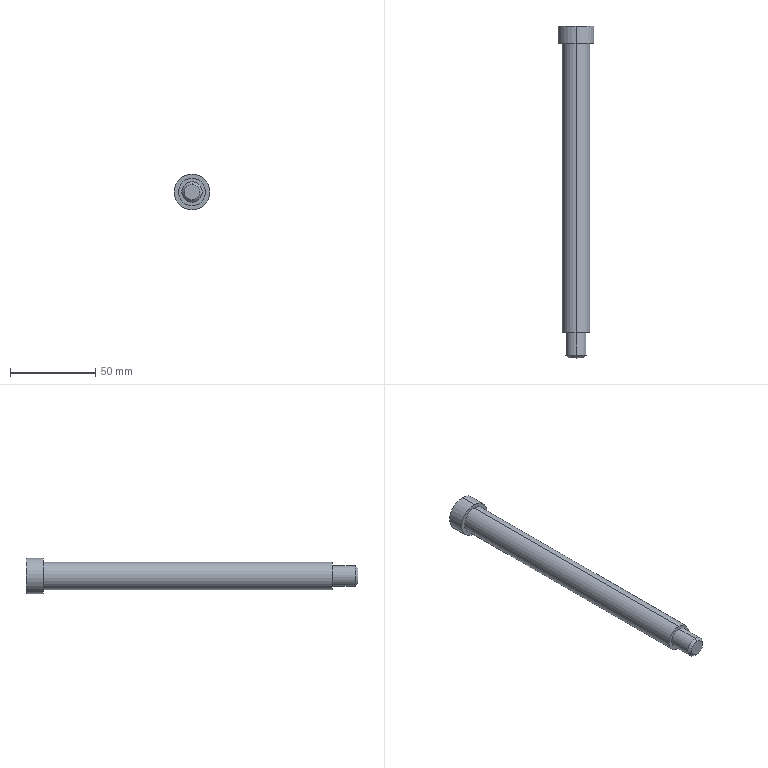Part | Creo | 1 solid | 19 faces | box 21 x 195 x 21 mm | volume 38969 mm3 | plane 11 | cylinder 6 | cone 2 | commonest cylinder face diameters 12 x2 16 x2 21 x2
STEP:
#1=CARTESIAN_POINT('',(0.2584,548.92,-30.381));
#2=VERTEX_POINT('',#1);
#3=CARTESIAN_POINT('',(4.258,548.92,-32.691));
#4=VERTEX_POINT('',#3);
#5=CARTESIAN_POINT('',(0.2584,548.92,-30.381));
#6=DIRECTION('',(0.866,0.,-0.5));
#7=VECTOR('',#6,4.619);
#8=LINE('',#5,#7);
#9=EDGE_CURVE('',#2,#4,#8,.T.);
#10=ORIENTED_EDGE('',*,*,#9,.F.);
#11=CARTESIAN_POINT('',(-3.742,548.92,-32.691));
#12=VERTEX_POINT('',#11);
#13=CARTESIAN_POINT('',(-3.742,548.92,-32.691));
#14=DIRECTION('',(0.866,0.,0.5));
#15=VECTOR('',#14,4.619);
#16=LINE('',#13,#15);
#17=EDGE_CURVE('',#12,#2,#16,.T.);
#18=ORIENTED_EDGE('',*,*,#17,.F.);
#19=CARTESIAN_POINT('',(-3.742,548.92,-37.309));
#20=VERTEX_POINT('',#19);
#21=CARTESIAN_POINT('',(-3.742,548.92,-32.691));
#22=DIRECTION('',(0.,0.,-1.));
#23=VECTOR('',#22,4.619);
#24=LINE('',#21,#23);
#25=EDGE_CURVE('',#12,#20,#24,.T.);
#26=ORIENTED_EDGE('',*,*,#25,.T.);
#27=CARTESIAN_POINT('',(0.2584,548.92,-39.619));
#28=VERTEX_POINT('',#27);
#29=CARTESIAN_POINT('',(0.2584,548.92,-39.619));
#30=DIRECTION('',(-0.866,0.,0.5));
#31=VECTOR('',#30,4.619);
#32=LINE('',#29,#31);
#33=EDGE_CURVE('',#28,#20,#32,.T.);
#34=ORIENTED_EDGE('',*,*,#33,.F.);
#35=CARTESIAN_POINT('',(4.258,548.92,-37.309));
#36=VERTEX_POINT('',#35);
#37=CARTESIAN_POINT('',(4.258,548.92,-37.309));
#38=DIRECTION('',(-0.866,0.,-0.5));
#39=VECTOR('',#38,4.619);
#40=LINE('',#37,#39);
#41=EDGE_CURVE('',#36,#28,#40,.T.);
#42=ORIENTED_EDGE('',*,*,#41,.F.);
#43=CARTESIAN_POINT('',(4.258,548.92,-37.309));
#44=DIRECTION('',(0.,0.,1.));
#45=VECTOR('',#44,4.619);
#46=LINE('',#43,#45);
#47=EDGE_CURVE('',#36,#4,#46,.T.);
#48=ORIENTED_EDGE('',*,*,#47,.T.);
#49=EDGE_LOOP('',(#10,#18,#26,#34,#42,#48));
#50=FACE_OUTER_BOUND('',#49,.F.);
#51=CARTESIAN_POINT('',(0.2584,548.92,-35.));
#52=DIRECTION('',(0.,1.,0.));
#53=DIRECTION('',(0.,0.,1.));
#54=AXIS2_PLACEMENT_3D('',#51,#52,#53);
#55=PLANE('',#54);
#56=ADVANCED_FACE('',(#50),#55,.T.);
#57=CARTESIAN_POINT('',(4.258,554.92,-32.691));
#58=VERTEX_POINT('',#57);
#59=CARTESIAN_POINT('',(4.258,548.92,-32.691));
#60=DIRECTION('',(0.,1.,0.));
#61=VECTOR('',#60,6.);
#62=LINE('',#59,#61);
#63=EDGE_CURVE('',#4,#58,#62,.T.);
#64=ORIENTED_EDGE('',*,*,#63,.T.);
#65=CARTESIAN_POINT('',(0.2584,554.92,-30.381));
#66=VERTEX_POINT('',#65);
#67=CARTESIAN_POINT('',(4.258,554.92,-32.691));
#68=DIRECTION('',(-0.866,0.,0.5));
#69=VECTOR('',#68,4.619);
#70=LINE('',#67,#69);
#71=EDGE_CURVE('',#58,#66,#70,.T.);
#72=ORIENTED_EDGE('',*,*,#71,.T.);
#73=CARTESIAN_POINT('',(0.2584,548.92,-30.381));
#74=DIRECTION('',(0.,1.,0.));
#75=VECTOR('',#74,6.);
#76=LINE('',#73,#75);
#77=EDGE_CURVE('',#2,#66,#76,.T.);
#78=ORIENTED_EDGE('',*,*,#77,.F.);
#79=ORIENTED_EDGE('',*,*,#9,.T.);
#80=EDGE_LOOP('',(#64,#72,#78,#79));
#81=FACE_OUTER_BOUND('',#80,.F.);
#82=CARTESIAN_POINT('',(0.2584,554.92,-30.381));
#83=DIRECTION('',(0.5,0.,0.866));
#84=DIRECTION('',(-0.866,0.,0.5));
#85=AXIS2_PLACEMENT_3D('',#82,#83,#84);
#86=PLANE('',#85);
#87=ADVANCED_FACE('',(#81),#86,.F.);
#88=CARTESIAN_POINT('',(4.258,554.92,-37.309));
#89=VERTEX_POINT('',#88);
#90=CARTESIAN_POINT('',(4.258,548.92,-37.309));
#91=DIRECTION('',(0.,1.,0.));
#92=VECTOR('',#91,6.);
#93=LINE('',#90,#92);
#94=EDGE_CURVE('',#36,#89,#93,.T.);
#95=ORIENTED_EDGE('',*,*,#94,.T.);
#96=CARTESIAN_POINT('',(4.258,554.92,-37.309));
#97=DIRECTION('',(0.,0.,1.));
#98=VECTOR('',#97,4.619);
#99=LINE('',#96,#98);
#100=EDGE_CURVE('',#89,#58,#99,.T.);
#101=ORIENTED_EDGE('',*,*,#100,.T.);
#102=ORIENTED_EDGE('',*,*,#63,.F.);
#103=ORIENTED_EDGE('',*,*,#47,.F.);
#104=EDGE_LOOP('',(#95,#101,#102,#103));
#105=FACE_OUTER_BOUND('',#104,.F.);
#106=CARTESIAN_POINT('',(4.258,554.92,-32.691));
#107=DIRECTION('',(1.,0.,0.));
#108=DIRECTION('',(0.,0.,1.));
#109=AXIS2_PLACEMENT_3D('',#106,#107,#108);
#110=PLANE('',#109);
#111=ADVANCED_FACE('',(#105),#110,.F.);
#112=CARTESIAN_POINT('',(0.2584,554.92,-39.619));
#113=VERTEX_POINT('',#112);
#114=CARTESIAN_POINT('',(0.2584,548.92,-39.619));
#115=DIRECTION('',(0.,1.,0.));
#116=VECTOR('',#115,6.);
#117=LINE('',#114,#116);
#118=EDGE_CURVE('',#28,#113,#117,.T.);
#119=ORIENTED_EDGE('',*,*,#118,.T.);
#120=CARTESIAN_POINT('',(0.2584,554.92,-39.619));
#121=DIRECTION('',(0.866,0.,0.5));
#122=VECTOR('',#121,4.619);
#123=LINE('',#120,#122);
#124=EDGE_CURVE('',#113,#89,#123,.T.);
#125=ORIENTED_EDGE('',*,*,#124,.T.);
#126=ORIENTED_EDGE('',*,*,#94,.F.);
#127=ORIENTED_EDGE('',*,*,#41,.T.);
#128=EDGE_LOOP('',(#119,#125,#126,#127));
#129=FACE_OUTER_BOUND('',#128,.F.);
#130=CARTESIAN_POINT('',(4.258,554.92,-37.309));
#131=DIRECTION('',(0.5,0.,-0.866));
#132=DIRECTION('',(0.866,0.,0.5));
#133=AXIS2_PLACEMENT_3D('',#130,#131,#132);
#134=PLANE('',#133);
#135=ADVANCED_FACE('',(#129),#134,.F.);
#136=CARTESIAN_POINT('',(-3.742,554.92,-37.309));
#137=VERTEX_POINT('',#136);
#138=CARTESIAN_POINT('',(-3.742,548.92,-37.309));
#139=DIRECTION('',(0.,1.,0.));
#140=VECTOR('',#139,6.);
#141=LINE('',#138,#140);
#142=EDGE_CURVE('',#20,#137,#141,.T.);
#143=ORIENTED_EDGE('',*,*,#142,.T.);
#144=CARTESIAN_POINT('',(-3.742,554.92,-37.309));
#145=DIRECTION('',(0.866,0.,-0.5));
#146=VECTOR('',#145,4.619);
#147=LINE('',#144,#146);
#148=EDGE_CURVE('',#137,#113,#147,.T.);
#149=ORIENTED_EDGE('',*,*,#148,.T.);
#150=ORIENTED_EDGE('',*,*,#118,.F.);
#151=ORIENTED_EDGE('',*,*,#33,.T.);
#152=EDGE_LOOP('',(#143,#149,#150,#151));
#153=FACE_OUTER_BOUND('',#152,.F.);
#154=CARTESIAN_POINT('',(0.2584,554.92,-39.619));
#155=DIRECTION('',(-0.5,0.,-0.866));
#156=DIRECTION('',(0.866,0.,-0.5));
#157=AXIS2_PLACEMENT_3D('',#154,#155,#156);
#158=PLANE('',#157);
#159=ADVANCED_FACE('',(#153),#158,.F.);
#160=CARTESIAN_POINT('',(-3.742,554.92,-32.691));
#161=VERTEX_POINT('',#160);
#162=CARTESIAN_POINT('',(-3.742,548.92,-32.691));
#163=DIRECTION('',(0.,1.,0.));
#164=VECTOR('',#163,6.);
#165=LINE('',#162,#164);
#166=EDGE_CURVE('',#12,#161,#165,.T.);
#167=ORIENTED_EDGE('',*,*,#166,.T.);
#168=CARTESIAN_POINT('',(-3.742,554.92,-32.691));
#169=DIRECTION('',(0.,0.,-1.));
#170=VECTOR('',#169,4.619);
#171=LINE('',#168,#170);
#172=EDGE_CURVE('',#161,#137,#171,.T.);
#173=ORIENTED_EDGE('',*,*,#172,.T.);
#174=ORIENTED_EDGE('',*,*,#142,.F.);
#175=ORIENTED_EDGE('',*,*,#25,.F.);
#176=EDGE_LOOP('',(#167,#173,#174,#175));
#177=FACE_OUTER_BOUND('',#176,.F.);
#178=CARTESIAN_POINT('',(-3.742,554.92,-37.309));
#179=DIRECTION('',(-1.,0.,0.));
#180=DIRECTION('',(0.,0.,-1.));
#181=AXIS2_PLACEMENT_3D('',#178,#179,#180);
#182=PLANE('',#181);
#183=ADVANCED_FACE('',(#177),#182,.F.);
#184=ORIENTED_EDGE('',*,*,#77,.T.);
#185=CARTESIAN_POINT('',(0.2584,554.92,-30.381));
#186=DIRECTION('',(-0.866,0.,-0.5));
#187=VECTOR('',#186,4.619);
#188=LINE('',#185,#187);
#189=EDGE_CURVE('',#66,#161,#188,.T.);
#190=ORIENTED_EDGE('',*,*,#189,.T.);
#191=ORIENTED_EDGE('',*,*,#166,.F.);
#192=ORIENTED_EDGE('',*,*,#17,.T.);
#193=EDGE_LOOP('',(#184,#190,#191,#192));
#194=FACE_OUTER_BOUND('',#193,.F.);
#195=CARTESIAN_POINT('',(-3.742,554.92,-32.691));
#196=DIRECTION('',(-0.5,0.,0.866));
#197=DIRECTION('',(-0.866,0.,-0.5));
#198=AXIS2_PLACEMENT_3D('',#195,#196,#197);
#199=PLANE('',#198);
#200=ADVANCED_FACE('',(#194),#199,.F.);
#201=CARTESIAN_POINT('',(0.2584,554.92,-24.5));
#202=VERTEX_POINT('',#201);
#203=CARTESIAN_POINT('',(0.2584,554.92,-45.5));
#204=VERTEX_POINT('',#203);
#205=CARTESIAN_POINT('',(0.2584,554.92,-35.));
#206=DIRECTION('',(0.,1.,0.));
#207=DIRECTION('',(0.,0.,1.));
#208=AXIS2_PLACEMENT_3D('',#205,#206,#207);
#209=CIRCLE('',#208,10.5);
#210=EDGE_CURVE('',#202,#204,#209,.T.);
#211=ORIENTED_EDGE('',*,*,#210,.F.);
#212=CARTESIAN_POINT('',(0.2584,554.92,-35.));
#213=DIRECTION('',(0.,1.,0.));
#214=DIRECTION('',(0.,0.,-1.));
#215=AXIS2_PLACEMENT_3D('',#212,#213,#214);
#216=CIRCLE('',#215,10.5);
#217=EDGE_CURVE('',#204,#202,#216,.T.);
#218=ORIENTED_EDGE('',*,*,#217,.F.);
#219=EDGE_LOOP('',(#211,#218));
#220=FACE_OUTER_BOUND('',#219,.F.);
#221=ORIENTED_EDGE('',*,*,#172,.F.);
#222=ORIENTED_EDGE('',*,*,#189,.F.);
#223=ORIENTED_EDGE('',*,*,#71,.F.);
#224=ORIENTED_EDGE('',*,*,#100,.F.);
#225=ORIENTED_EDGE('',*,*,#124,.F.);
#226=ORIENTED_EDGE('',*,*,#148,.F.);
#227=EDGE_LOOP('',(#221,#222,#223,#224,#225,#226));
#228=FACE_BOUND('',#227,.F.);
#229=CARTESIAN_POINT('',(0.2584,554.92,-35.));
#230=DIRECTION('',(0.,-1.,0.));
#231=DIRECTION('',(0.,0.,-1.));
#232=AXIS2_PLACEMENT_3D('',#229,#230,#231);
#233=PLANE('',#232);
#234=ADVANCED_FACE('',(#220,#228),#233,.F.);
#235=CARTESIAN_POINT('',(0.2584,544.92,-45.5));
#236=VERTEX_POINT('',#235);
#237=CARTESIAN_POINT('',(0.2584,544.92,-24.5));
#238=VERTEX_POINT('',#237);
#239=CARTESIAN_POINT('',(0.2584,544.92,-35.));
#240=DIRECTION('',(0.,-1.,0.));
#241=DIRECTION('',(0.,0.,-1.));
#242=AXIS2_PLACEMENT_3D('',#239,#240,#241);
#243=CIRCLE('',#242,10.5);
#244=EDGE_CURVE('',#236,#238,#243,.T.);
#245=ORIENTED_EDGE('',*,*,#244,.T.);
#246=CARTESIAN_POINT('',(0.2584,554.92,-24.5));
#247=DIRECTION('',(0.,-1.,0.));
#248=VECTOR('',#247,10.);
#249=LINE('',#246,#248);
#250=EDGE_CURVE('',#202,#238,#249,.T.);
#251=ORIENTED_EDGE('',*,*,#250,.F.);
#252=ORIENTED_EDGE('',*,*,#210,.T.);
#253=CARTESIAN_POINT('',(0.2584,554.92,-45.5));
#254=DIRECTION('',(0.,-1.,0.));
#255=VECTOR('',#254,10.);
#256=LINE('',#253,#255);
#257=EDGE_CURVE('',#204,#236,#256,.T.);
#258=ORIENTED_EDGE('',*,*,#257,.T.);
#259=EDGE_LOOP('',(#245,#251,#252,#258));
#260=FACE_OUTER_BOUND('',#259,.F.);
#261=CARTESIAN_POINT('',(0.2584,562.17,-35.));
#262=DIRECTION('',(0.,-1.,0.));
#263=DIRECTION('',(0.,0.,-1.));
#264=AXIS2_PLACEMENT_3D('',#261,#262,#263);
#265=CYLINDRICAL_SURFACE('',#264,10.5);
#266=ADVANCED_FACE('',(#260),#265,.T.);
#267=CARTESIAN_POINT('',(0.2584,544.92,-35.));
#268=DIRECTION('',(0.,-1.,0.));
#269=DIRECTION('',(0.,0.,1.));
#270=AXIS2_PLACEMENT_3D('',#267,#268,#269);
#271=CIRCLE('',#270,10.5);
#272=EDGE_CURVE('',#238,#236,#271,.T.);
#273=ORIENTED_EDGE('',*,*,#272,.F.);
#274=ORIENTED_EDGE('',*,*,#244,.F.);
#275=EDGE_LOOP('',(#273,#274));
#276=FACE_OUTER_BOUND('',#275,.F.);
#277=CARTESIAN_POINT('',(0.2584,544.92,-27.));
#278=VERTEX_POINT('',#277);
#279=CARTESIAN_POINT('',(0.2584,544.92,-43.));
#280=VERTEX_POINT('',#279);
#281=CARTESIAN_POINT('',(0.2584,544.92,-35.));
#282=DIRECTION('',(0.,1.,0.));
#283=DIRECTION('',(0.,0.,1.));
#284=AXIS2_PLACEMENT_3D('',#281,#282,#283);
#285=CIRCLE('',#284,8.);
#286=EDGE_CURVE('',#278,#280,#285,.T.);
#287=ORIENTED_EDGE('',*,*,#286,.F.);
#288=CARTESIAN_POINT('',(0.2584,544.92,-35.));
#289=DIRECTION('',(0.,1.,0.));
#290=DIRECTION('',(0.,0.,-1.));
#291=AXIS2_PLACEMENT_3D('',#288,#289,#290);
#292=CIRCLE('',#291,8.);
#293=EDGE_CURVE('',#280,#278,#292,.T.);
#294=ORIENTED_EDGE('',*,*,#293,.F.);
#295=EDGE_LOOP('',(#287,#294));
#296=FACE_BOUND('',#295,.F.);
#297=CARTESIAN_POINT('',(0.2584,544.92,-35.));
#298=DIRECTION('',(0.,-1.,0.));
#299=DIRECTION('',(0.,0.,-1.));
#300=AXIS2_PLACEMENT_3D('',#297,#298,#299);
#301=PLANE('',#300);
#302=ADVANCED_FACE('',(#276,#296),#301,.T.);
#303=CARTESIAN_POINT('',(0.2584,374.92,-43.));
#304=VERTEX_POINT('',#303);
#305=CARTESIAN_POINT('',(0.2584,374.92,-27.));
#306=VERTEX_POINT('',#305);
#307=CARTESIAN_POINT('',(0.2584,374.92,-35.));
#308=DIRECTION('',(0.,-1.,0.));
#309=DIRECTION('',(0.,0.,-1.));
#310=AXIS2_PLACEMENT_3D('',#307,#308,#309);
#311=CIRCLE('',#310,8.);
#312=EDGE_CURVE('',#304,#306,#311,.T.);
#313=ORIENTED_EDGE('',*,*,#312,.T.);
#314=CARTESIAN_POINT('',(0.2584,544.92,-27.));
#315=DIRECTION('',(0.,-1.,0.));
#316=VECTOR('',#315,170.);
#317=LINE('',#314,#316);
#318=EDGE_CURVE('',#278,#306,#317,.T.);
#319=ORIENTED_EDGE('',*,*,#318,.F.);
#320=ORIENTED_EDGE('',*,*,#286,.T.);
#321=CARTESIAN_POINT('',(0.2584,544.92,-43.));
#322=DIRECTION('',(0.,-1.,0.));
#323=VECTOR('',#322,170.);
#324=LINE('',#321,#323);
#325=EDGE_CURVE('',#280,#304,#324,.T.);
#326=ORIENTED_EDGE('',*,*,#325,.T.);
#327=EDGE_LOOP('',(#313,#319,#320,#326));
#328=FACE_OUTER_BOUND('',#327,.F.);
#329=CARTESIAN_POINT('',(0.2584,512.17,-35.));
#330=DIRECTION('',(0.,-1.,0.));
#331=DIRECTION('',(0.,0.,-1.));
#332=AXIS2_PLACEMENT_3D('',#329,#330,#331);
#333=CYLINDRICAL_SURFACE('',#332,8.);
#334=ADVANCED_FACE('',(#328),#333,.T.);
#335=CARTESIAN_POINT('',(0.2584,374.92,-35.));
#336=DIRECTION('',(0.,-1.,0.));
#337=DIRECTION('',(0.,0.,1.));
#338=AXIS2_PLACEMENT_3D('',#335,#336,#337);
#339=CIRCLE('',#338,8.);
#340=EDGE_CURVE('',#306,#304,#339,.T.);
#341=ORIENTED_EDGE('',*,*,#340,.F.);
#342=ORIENTED_EDGE('',*,*,#312,.F.);
#343=EDGE_LOOP('',(#341,#342));
#344=FACE_OUTER_BOUND('',#343,.F.);
#345=CARTESIAN_POINT('',(0.2584,374.92,-29.));
#346=VERTEX_POINT('',#345);
#347=CARTESIAN_POINT('',(0.2584,374.92,-41.));
#348=VERTEX_POINT('',#347);
#349=CARTESIAN_POINT('',(0.2584,374.92,-35.));
#350=DIRECTION('',(0.,1.,0.));
#351=DIRECTION('',(0.,0.,1.));
#352=AXIS2_PLACEMENT_3D('',#349,#350,#351);
#353=CIRCLE('',#352,6.);
#354=EDGE_CURVE('',#346,#348,#353,.T.);
#355=ORIENTED_EDGE('',*,*,#354,.F.);
#356=CARTESIAN_POINT('',(0.2584,374.92,-35.));
#357=DIRECTION('',(0.,1.,0.));
#358=DIRECTION('',(0.,0.,-1.));
#359=AXIS2_PLACEMENT_3D('',#356,#357,#358);
#360=CIRCLE('',#359,6.);
#361=EDGE_CURVE('',#348,#346,#360,.T.);
#362=ORIENTED_EDGE('',*,*,#361,.F.);
#363=EDGE_LOOP('',(#355,#362));
#364=FACE_BOUND('',#363,.F.);
#365=CARTESIAN_POINT('',(0.2584,374.92,-35.));
#366=DIRECTION('',(0.,-1.,0.));
#367=DIRECTION('',(0.,0.,-1.));
#368=AXIS2_PLACEMENT_3D('',#365,#366,#367);
#369=PLANE('',#368);
#370=ADVANCED_FACE('',(#344,#364),#369,.T.);
#371=CARTESIAN_POINT('',(0.2584,361.42,-41.));
#372=VERTEX_POINT('',#371);
#373=CARTESIAN_POINT('',(0.2584,361.42,-29.));
#374=VERTEX_POINT('',#373);
#375=CARTESIAN_POINT('',(0.2584,361.42,-35.));
#376=DIRECTION('',(0.,-1.,0.));
#377=DIRECTION('',(0.,0.,-1.));
#378=AXIS2_PLACEMENT_3D('',#375,#376,#377);
#379=CIRCLE('',#378,6.);
#380=EDGE_CURVE('',#372,#374,#379,.T.);
#381=ORIENTED_EDGE('',*,*,#380,.T.);
#382=CARTESIAN_POINT('',(0.2584,374.92,-29.));
#383=DIRECTION('',(0.,-1.,0.));
#384=VECTOR('',#383,13.5);
#385=LINE('',#382,#384);
#386=EDGE_CURVE('',#346,#374,#385,.T.);
#387=ORIENTED_EDGE('',*,*,#386,.F.);
#388=ORIENTED_EDGE('',*,*,#354,.T.);
#389=CARTESIAN_POINT('',(0.2584,374.92,-41.));
#390=DIRECTION('',(0.,-1.,0.));
#391=VECTOR('',#390,13.5);
#392=LINE('',#389,#391);
#393=EDGE_CURVE('',#348,#372,#392,.T.);
#394=ORIENTED_EDGE('',*,*,#393,.T.);
#395=EDGE_LOOP('',(#381,#387,#388,#394));
#396=FACE_OUTER_BOUND('',#395,.F.);
#397=CARTESIAN_POINT('',(0.2584,512.17,-35.));
#398=DIRECTION('',(0.,-1.,0.));
#399=DIRECTION('',(0.,0.,-1.));
#400=AXIS2_PLACEMENT_3D('',#397,#398,#399);
#401=CYLINDRICAL_SURFACE('',#400,6.);
#402=ADVANCED_FACE('',(#396),#401,.T.);
#403=CARTESIAN_POINT('',(0.2584,359.92,-39.5));
#404=VERTEX_POINT('',#403);
#405=CARTESIAN_POINT('',(0.2584,359.92,-30.5));
#406=VERTEX_POINT('',#405);
#407=CARTESIAN_POINT('',(0.2584,359.92,-35.));
#408=DIRECTION('',(0.,-1.,0.));
#409=DIRECTION('',(0.,0.,-1.));
#410=AXIS2_PLACEMENT_3D('',#407,#408,#409);
#411=CIRCLE('',#410,4.5);
#412=EDGE_CURVE('',#404,#406,#411,.T.);
#413=ORIENTED_EDGE('',*,*,#412,.T.);
#414=CARTESIAN_POINT('',(0.2584,359.92,-30.5));
#415=DIRECTION('',(0.,0.7071,0.7071));
#416=VECTOR('',#415,2.121);
#417=LINE('',#414,#416);
#418=EDGE_CURVE('',#406,#374,#417,.T.);
#419=ORIENTED_EDGE('',*,*,#418,.T.);
#420=ORIENTED_EDGE('',*,*,#380,.F.);
#421=CARTESIAN_POINT('',(0.2584,359.92,-39.5));
#422=DIRECTION('',(0.,0.7071,-0.7071));
#423=VECTOR('',#422,2.121);
#424=LINE('',#421,#423);
#425=EDGE_CURVE('',#404,#372,#424,.T.);
#426=ORIENTED_EDGE('',*,*,#425,.F.);
#427=EDGE_LOOP('',(#413,#419,#420,#426));
#428=FACE_OUTER_BOUND('',#427,.F.);
#429=CARTESIAN_POINT('',(0.2584,360.67,-35.));
#430=DIRECTION('',(0.,1.,0.));
#431=DIRECTION('',(0.,0.,1.));
#432=AXIS2_PLACEMENT_3D('',#429,#430,#431);
#433=CONICAL_SURFACE('',#432,5.25,45.);
#434=ADVANCED_FACE('',(#428),#433,.T.);
#435=CARTESIAN_POINT('',(0.2584,359.92,-35.));
#436=DIRECTION('',(0.,-1.,0.));
#437=DIRECTION('',(0.,0.,1.));
#438=AXIS2_PLACEMENT_3D('',#435,#436,#437);
#439=CIRCLE('',#438,4.5);
#440=EDGE_CURVE('',#406,#404,#439,.T.);
#441=ORIENTED_EDGE('',*,*,#440,.F.);
#442=ORIENTED_EDGE('',*,*,#412,.F.);
#443=EDGE_LOOP('',(#441,#442));
#444=FACE_OUTER_BOUND('',#443,.F.);
#445=CARTESIAN_POINT('',(0.2584,359.92,-35.));
#446=DIRECTION('',(0.,-1.,0.));
#447=DIRECTION('',(0.,0.,-1.));
#448=AXIS2_PLACEMENT_3D('',#445,#446,#447);
#449=PLANE('',#448);
#450=ADVANCED_FACE('',(#444),#449,.T.);
#451=ORIENTED_EDGE('',*,*,#440,.T.);
#452=ORIENTED_EDGE('',*,*,#425,.T.);
#453=CARTESIAN_POINT('',(0.2584,361.42,-35.));
#454=DIRECTION('',(0.,-1.,0.));
#455=DIRECTION('',(0.,0.,1.));
#456=AXIS2_PLACEMENT_3D('',#453,#454,#455);
#457=CIRCLE('',#456,6.);
#458=EDGE_CURVE('',#374,#372,#457,.T.);
#459=ORIENTED_EDGE('',*,*,#458,.F.);
#460=ORIENTED_EDGE('',*,*,#418,.F.);
#461=EDGE_LOOP('',(#451,#452,#459,#460));
#462=FACE_OUTER_BOUND('',#461,.F.);
#463=CARTESIAN_POINT('',(0.2584,360.67,-35.));
#464=DIRECTION('',(0.,1.,0.));
#465=DIRECTION('',(0.,0.,1.));
#466=AXIS2_PLACEMENT_3D('',#463,#464,#465);
#467=CONICAL_SURFACE('',#466,5.25,45.);
#468=ADVANCED_FACE('',(#462),#467,.T.);
#469=ORIENTED_EDGE('',*,*,#458,.T.);
#470=ORIENTED_EDGE('',*,*,#393,.F.);
#471=ORIENTED_EDGE('',*,*,#361,.T.);
#472=ORIENTED_EDGE('',*,*,#386,.T.);
#473=EDGE_LOOP('',(#469,#470,#471,#472));
#474=FACE_OUTER_BOUND('',#473,.F.);
#475=CARTESIAN_POINT('',(0.2584,512.17,-35.));
#476=DIRECTION('',(0.,-1.,0.));
#477=DIRECTION('',(0.,0.,-1.));
#478=AXIS2_PLACEMENT_3D('',#475,#476,#477);
#479=CYLINDRICAL_SURFACE('',#478,6.);
#480=ADVANCED_FACE('',(#474),#479,.T.);
#481=ORIENTED_EDGE('',*,*,#340,.T.);
#482=ORIENTED_EDGE('',*,*,#325,.F.);
#483=ORIENTED_EDGE('',*,*,#293,.T.);
#484=ORIENTED_EDGE('',*,*,#318,.T.);
#485=EDGE_LOOP('',(#481,#482,#483,#484));
#486=FACE_OUTER_BOUND('',#485,.F.);
#487=CARTESIAN_POINT('',(0.2584,512.17,-35.));
#488=DIRECTION('',(0.,-1.,0.));
#489=DIRECTION('',(0.,0.,-1.));
#490=AXIS2_PLACEMENT_3D('',#487,#488,#489);
#491=CYLINDRICAL_SURFACE('',#490,8.);
#492=ADVANCED_FACE('',(#486),#491,.T.);
#493=ORIENTED_EDGE('',*,*,#272,.T.);
#494=ORIENTED_EDGE('',*,*,#257,.F.);
#495=ORIENTED_EDGE('',*,*,#217,.T.);
#496=ORIENTED_EDGE('',*,*,#250,.T.);
#497=EDGE_LOOP('',(#493,#494,#495,#496));
#498=FACE_OUTER_BOUND('',#497,.F.);
#499=CARTESIAN_POINT('',(0.2584,562.17,-35.));
#500=DIRECTION('',(0.,-1.,0.));
#501=DIRECTION('',(0.,0.,-1.));
#502=AXIS2_PLACEMENT_3D('',#499,#500,#501);
#503=CYLINDRICAL_SURFACE('',#502,10.5);
#504=ADVANCED_FACE('',(#498),#503,.T.);
#505=CLOSED_SHELL('',(#56,#87,#111,#135,#159,#183,#200,#234,#266,#302,#334,#370,#402,#434,#450,#468,#480,#492,#504));
#506=MANIFOLD_SOLID_BREP('',#505);
#507=(LENGTH_UNIT()NAMED_UNIT(*)SI_UNIT(.MILLI.,.METRE.));
#508=UNCERTAINTY_MEASURE_WITH_UNIT(LENGTH_MEASURE(0.01972),#507,'','');
#509=(NAMED_UNIT(*)PLANE_ANGLE_UNIT()SI_UNIT($,.RADIAN.));
#510=PLANE_ANGLE_MEASURE_WITH_UNIT(PLANE_ANGLE_MEASURE(0.01745),#509);
#511=(CONVERSION_BASED_UNIT('DEGREE',#510)NAMED_UNIT(*)PLANE_ANGLE_UNIT());
#512=(NAMED_UNIT(*)SI_UNIT($,.STERADIAN.)SOLID_ANGLE_UNIT());
#513=(GEOMETRIC_REPRESENTATION_CONTEXT(3)GLOBAL_UNCERTAINTY_ASSIGNED_CONTEXT((#508))GLOBAL_UNIT_ASSIGNED_CONTEXT((#507,#511,#512))REPRESENTATION_CONTEXT('',''));
#514=ADVANCED_BREP_SHAPE_REPRESENTATION('',(#506),#513);